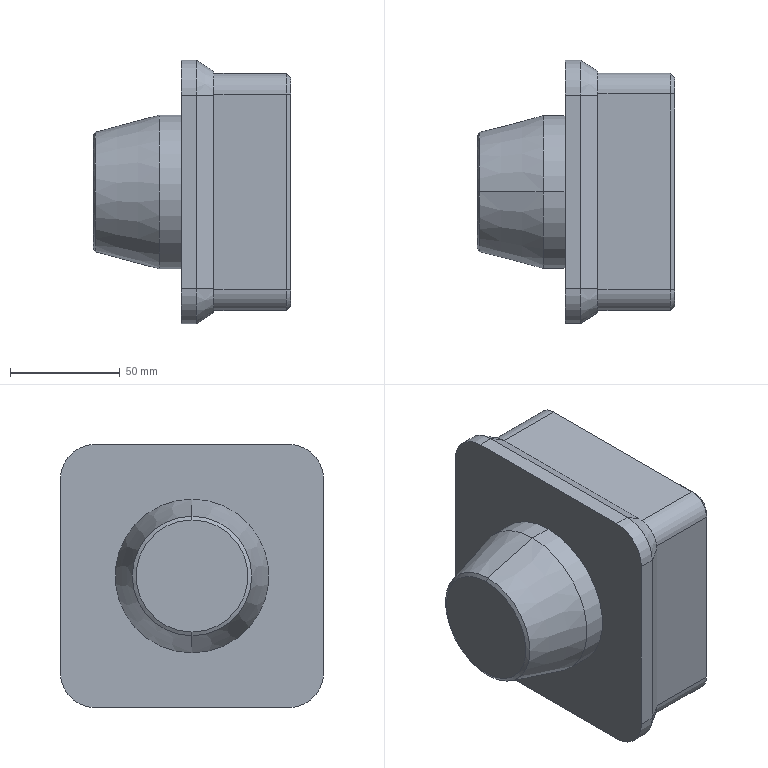Part | SolidWorks | features Chamfer 3, ICE 2, Revolution 1 | 1 solid | 42 faces | box 90 x 120 x 120 mm | volume 737957 mm3 | plane 20 | cone 12 | cylinder 10 | commonest cylinder face diameters 18.818 x4 32 x4 70 x2
STEP:
#1=CARTESIAN_POINT('',(0.,0.,25.547));
#2=VERTEX_POINT('',#1);
#3=CARTESIAN_POINT('',(0.,0.,-25.547));
#4=VERTEX_POINT('',#3);
#5=CARTESIAN_POINT('',(0.,0.,0.));
#6=DIRECTION('',(-1.,0.,0.));
#7=DIRECTION('',(0.,0.,1.));
#8=AXIS2_PLACEMENT_3D('',#5,#6,#7);
#9=CIRCLE('',#8,25.547);
#10=EDGE_CURVE('',#2,#4,#9,.T.);
#11=ORIENTED_EDGE('',*,*,#10,.F.);
#12=CARTESIAN_POINT('',(0.9659,0.,27.22));
#13=VERTEX_POINT('',#12);
#14=CARTESIAN_POINT('',(0.,0.,25.547));
#15=DIRECTION('',(0.5,0.,0.866));
#16=VECTOR('',#15,1000.);
#17=LINE('',#14,#16);
#18=EDGE_CURVE('',#2,#13,#17,.T.);
#19=ORIENTED_EDGE('',*,*,#18,.T.);
#20=CARTESIAN_POINT('',(0.9659,0.,-27.22));
#21=VERTEX_POINT('',#20);
#22=CARTESIAN_POINT('',(0.9659,0.,0.));
#23=DIRECTION('',(1.,0.,0.));
#24=DIRECTION('',(0.,0.,-1.));
#25=AXIS2_PLACEMENT_3D('',#22,#23,#24);
#26=CIRCLE('',#25,27.22);
#27=EDGE_CURVE('',#21,#13,#26,.T.);
#28=ORIENTED_EDGE('',*,*,#27,.F.);
#29=CARTESIAN_POINT('',(0.,0.,-25.547));
#30=DIRECTION('',(0.5,0.,-0.866));
#31=VECTOR('',#30,1000.);
#32=LINE('',#29,#31);
#33=EDGE_CURVE('',#4,#21,#32,.T.);
#34=ORIENTED_EDGE('',*,*,#33,.F.);
#35=EDGE_LOOP('',(#11,#19,#28,#34));
#36=FACE_OUTER_BOUND('',#35,.T.);
#37=CARTESIAN_POINT('',(0.,0.,0.));
#38=DIRECTION('',(1.,0.,0.));
#39=DIRECTION('',(0.,0.,-1.));
#40=AXIS2_PLACEMENT_3D('',#37,#38,#39);
#41=CONICAL_SURFACE('',#40,25.547,1.047);
#42=ADVANCED_FACE('',(#36),#41,.T.);
#43=ORIENTED_EDGE('',*,*,#27,.T.);
#44=CARTESIAN_POINT('',(30.,0.,35.));
#45=VERTEX_POINT('',#44);
#46=CARTESIAN_POINT('',(30.,0.,35.));
#47=DIRECTION('',(0.9659,0.,0.2588));
#48=VECTOR('',#47,1000.);
#49=LINE('',#46,#48);
#50=EDGE_CURVE('',#13,#45,#49,.T.);
#51=ORIENTED_EDGE('',*,*,#50,.T.);
#52=CARTESIAN_POINT('',(30.,0.,-35.));
#53=VERTEX_POINT('',#52);
#54=CARTESIAN_POINT('',(30.,0.,0.));
#55=DIRECTION('',(-1.,0.,0.));
#56=DIRECTION('',(0.,0.,1.));
#57=AXIS2_PLACEMENT_3D('',#54,#55,#56);
#58=CIRCLE('',#57,35.);
#59=EDGE_CURVE('',#45,#53,#58,.T.);
#60=ORIENTED_EDGE('',*,*,#59,.T.);
#61=CARTESIAN_POINT('',(30.,0.,-35.));
#62=DIRECTION('',(0.9659,0.,-0.2588));
#63=VECTOR('',#62,1000.);
#64=LINE('',#61,#63);
#65=EDGE_CURVE('',#21,#53,#64,.T.);
#66=ORIENTED_EDGE('',*,*,#65,.F.);
#67=EDGE_LOOP('',(#43,#51,#60,#66));
#68=FACE_OUTER_BOUND('',#67,.T.);
#69=CARTESIAN_POINT('',(30.,0.,0.));
#70=DIRECTION('',(1.,0.,0.));
#71=DIRECTION('',(0.,0.,-1.));
#72=AXIS2_PLACEMENT_3D('',#69,#70,#71);
#73=CONICAL_SURFACE('',#72,35.,0.2618);
#74=ADVANCED_FACE('',(#68),#73,.T.);
#75=CARTESIAN_POINT('',(40.,0.,35.));
#76=VERTEX_POINT('',#75);
#77=CARTESIAN_POINT('',(40.,0.,-35.));
#78=VERTEX_POINT('',#77);
#79=CARTESIAN_POINT('',(40.,0.,0.));
#80=DIRECTION('',(-1.,0.,0.));
#81=DIRECTION('',(0.,0.,1.));
#82=AXIS2_PLACEMENT_3D('',#79,#80,#81);
#83=CIRCLE('',#82,35.);
#84=EDGE_CURVE('',#76,#78,#83,.T.);
#85=ORIENTED_EDGE('',*,*,#84,.T.);
#86=CARTESIAN_POINT('',(0.,0.,-35.));
#87=DIRECTION('',(-1.,0.,0.));
#88=VECTOR('',#87,1000.);
#89=LINE('',#86,#88);
#90=EDGE_CURVE('',#78,#53,#89,.T.);
#91=ORIENTED_EDGE('',*,*,#90,.T.);
#92=ORIENTED_EDGE('',*,*,#59,.F.);
#93=CARTESIAN_POINT('',(0.,0.,35.));
#94=DIRECTION('',(-1.,0.,0.));
#95=VECTOR('',#94,1000.);
#96=LINE('',#93,#95);
#97=EDGE_CURVE('',#76,#45,#96,.T.);
#98=ORIENTED_EDGE('',*,*,#97,.F.);
#99=EDGE_LOOP('',(#85,#91,#92,#98));
#100=FACE_OUTER_BOUND('',#99,.T.);
#101=CARTESIAN_POINT('',(0.,0.,0.));
#102=DIRECTION('',(-1.,0.,0.));
#103=DIRECTION('',(0.,0.,1.));
#104=AXIS2_PLACEMENT_3D('',#101,#102,#103);
#105=CYLINDRICAL_SURFACE('',#104,35.);
#106=ADVANCED_FACE('',(#100),#105,.T.);
#107=CARTESIAN_POINT('',(55.,55.,44.));
#108=VERTEX_POINT('',#107);
#109=CARTESIAN_POINT('',(55.,44.,55.));
#110=VERTEX_POINT('',#109);
#111=CARTESIAN_POINT('',(55.,44.,44.));
#112=DIRECTION('',(1.,0.,0.));
#113=DIRECTION('',(0.,0.,1.));
#114=AXIS2_PLACEMENT_3D('',#111,#112,#113);
#115=CIRCLE('',#114,11.);
#116=EDGE_CURVE('',#108,#110,#115,.T.);
#117=ORIENTED_EDGE('',*,*,#116,.T.);
#118=CARTESIAN_POINT('',(55.,-44.,55.));
#119=VERTEX_POINT('',#118);
#120=CARTESIAN_POINT('',(55.,-44.,55.));
#121=DIRECTION('',(0.,-1.,0.));
#122=VECTOR('',#121,1000.);
#123=LINE('',#120,#122);
#124=EDGE_CURVE('',#110,#119,#123,.T.);
#125=ORIENTED_EDGE('',*,*,#124,.T.);
#126=CARTESIAN_POINT('',(55.,-55.,44.));
#127=VERTEX_POINT('',#126);
#128=CARTESIAN_POINT('',(55.,-44.,44.));
#129=DIRECTION('',(1.,0.,0.));
#130=DIRECTION('',(0.,0.,1.));
#131=AXIS2_PLACEMENT_3D('',#128,#129,#130);
#132=CIRCLE('',#131,11.);
#133=EDGE_CURVE('',#119,#127,#132,.T.);
#134=ORIENTED_EDGE('',*,*,#133,.T.);
#135=CARTESIAN_POINT('',(55.,-55.,-44.));
#136=VERTEX_POINT('',#135);
#137=CARTESIAN_POINT('',(55.,-55.,44.));
#138=DIRECTION('',(0.,0.,-1.));
#139=VECTOR('',#138,1000.);
#140=LINE('',#137,#139);
#141=EDGE_CURVE('',#127,#136,#140,.T.);
#142=ORIENTED_EDGE('',*,*,#141,.T.);
#143=CARTESIAN_POINT('',(55.,-44.,-55.));
#144=VERTEX_POINT('',#143);
#145=CARTESIAN_POINT('',(55.,-44.,-44.));
#146=DIRECTION('',(1.,0.,0.));
#147=DIRECTION('',(0.,0.,1.));
#148=AXIS2_PLACEMENT_3D('',#145,#146,#147);
#149=CIRCLE('',#148,11.);
#150=EDGE_CURVE('',#136,#144,#149,.T.);
#151=ORIENTED_EDGE('',*,*,#150,.T.);
#152=CARTESIAN_POINT('',(55.,44.,-55.));
#153=VERTEX_POINT('',#152);
#154=CARTESIAN_POINT('',(55.,-44.,-55.));
#155=DIRECTION('',(0.,1.,0.));
#156=VECTOR('',#155,1000.);
#157=LINE('',#154,#156);
#158=EDGE_CURVE('',#144,#153,#157,.T.);
#159=ORIENTED_EDGE('',*,*,#158,.T.);
#160=CARTESIAN_POINT('',(55.,55.,-44.));
#161=VERTEX_POINT('',#160);
#162=CARTESIAN_POINT('',(55.,44.,-44.));
#163=DIRECTION('',(1.,0.,0.));
#164=DIRECTION('',(0.,0.,1.));
#165=AXIS2_PLACEMENT_3D('',#162,#163,#164);
#166=CIRCLE('',#165,11.);
#167=EDGE_CURVE('',#153,#161,#166,.T.);
#168=ORIENTED_EDGE('',*,*,#167,.T.);
#169=CARTESIAN_POINT('',(55.,55.,44.));
#170=DIRECTION('',(0.,0.,1.));
#171=VECTOR('',#170,1000.);
#172=LINE('',#169,#171);
#173=EDGE_CURVE('',#161,#108,#172,.T.);
#174=ORIENTED_EDGE('',*,*,#173,.T.);
#175=EDGE_LOOP('',(#117,#125,#134,#142,#151,#159,#168,#174));
#176=FACE_OUTER_BOUND('',#175,.T.);
#177=CARTESIAN_POINT('',(55.,44.591,-54.));
#178=VERTEX_POINT('',#177);
#179=CARTESIAN_POINT('',(55.,54.,-44.591));
#180=VERTEX_POINT('',#179);
#181=CARTESIAN_POINT('',(55.,44.591,-44.591));
#182=DIRECTION('',(1.,0.,0.));
#183=DIRECTION('',(0.,0.,1.));
#184=AXIS2_PLACEMENT_3D('',#181,#182,#183);
#185=CIRCLE('',#184,9.409);
#186=EDGE_CURVE('',#178,#180,#185,.T.);
#187=ORIENTED_EDGE('',*,*,#186,.F.);
#188=CARTESIAN_POINT('',(55.,-44.591,-54.));
#189=VERTEX_POINT('',#188);
#190=CARTESIAN_POINT('',(55.,-44.591,-54.));
#191=DIRECTION('',(0.,1.,0.));
#192=VECTOR('',#191,1000.);
#193=LINE('',#190,#192);
#194=EDGE_CURVE('',#189,#178,#193,.T.);
#195=ORIENTED_EDGE('',*,*,#194,.F.);
#196=CARTESIAN_POINT('',(55.,-54.,-44.591));
#197=VERTEX_POINT('',#196);
#198=CARTESIAN_POINT('',(55.,-44.591,-44.591));
#199=DIRECTION('',(1.,0.,0.));
#200=DIRECTION('',(0.,0.,1.));
#201=AXIS2_PLACEMENT_3D('',#198,#199,#200);
#202=CIRCLE('',#201,9.409);
#203=EDGE_CURVE('',#197,#189,#202,.T.);
#204=ORIENTED_EDGE('',*,*,#203,.F.);
#205=CARTESIAN_POINT('',(55.,-54.,44.591));
#206=VERTEX_POINT('',#205);
#207=CARTESIAN_POINT('',(55.,-54.,44.591));
#208=DIRECTION('',(0.,0.,-1.));
#209=VECTOR('',#208,1000.);
#210=LINE('',#207,#209);
#211=EDGE_CURVE('',#206,#197,#210,.T.);
#212=ORIENTED_EDGE('',*,*,#211,.F.);
#213=CARTESIAN_POINT('',(55.,-44.591,54.));
#214=VERTEX_POINT('',#213);
#215=CARTESIAN_POINT('',(55.,-44.591,44.591));
#216=DIRECTION('',(1.,0.,0.));
#217=DIRECTION('',(0.,0.,1.));
#218=AXIS2_PLACEMENT_3D('',#215,#216,#217);
#219=CIRCLE('',#218,9.409);
#220=EDGE_CURVE('',#214,#206,#219,.T.);
#221=ORIENTED_EDGE('',*,*,#220,.F.);
#222=CARTESIAN_POINT('',(55.,44.591,54.));
#223=VERTEX_POINT('',#222);
#224=CARTESIAN_POINT('',(55.,-44.591,54.));
#225=DIRECTION('',(0.,-1.,0.));
#226=VECTOR('',#225,1000.);
#227=LINE('',#224,#226);
#228=EDGE_CURVE('',#223,#214,#227,.T.);
#229=ORIENTED_EDGE('',*,*,#228,.F.);
#230=CARTESIAN_POINT('',(55.,54.,44.591));
#231=VERTEX_POINT('',#230);
#232=CARTESIAN_POINT('',(55.,44.591,44.591));
#233=DIRECTION('',(1.,0.,0.));
#234=DIRECTION('',(0.,0.,1.));
#235=AXIS2_PLACEMENT_3D('',#232,#233,#234);
#236=CIRCLE('',#235,9.409);
#237=EDGE_CURVE('',#231,#223,#236,.T.);
#238=ORIENTED_EDGE('',*,*,#237,.F.);
#239=CARTESIAN_POINT('',(55.,54.,44.591));
#240=DIRECTION('',(0.,0.,1.));
#241=VECTOR('',#240,1000.);
#242=LINE('',#239,#241);
#243=EDGE_CURVE('',#180,#231,#242,.T.);
#244=ORIENTED_EDGE('',*,*,#243,.F.);
#245=EDGE_LOOP('',(#187,#195,#204,#212,#221,#229,#238,#244));
#246=FACE_BOUND('',#245,.T.);
#247=CARTESIAN_POINT('',(55.,-44.,44.));
#248=DIRECTION('',(-1.,0.,0.));
#249=DIRECTION('',(0.,0.,1.));
#250=AXIS2_PLACEMENT_3D('',#247,#248,#249);
#251=PLANE('',#250);
#252=ADVANCED_FACE('',(#176,#246),#251,.F.);
#253=ORIENTED_EDGE('',*,*,#90,.F.);
#254=CARTESIAN_POINT('',(40.,0.,0.));
#255=DIRECTION('',(-1.,0.,0.));
#256=DIRECTION('',(0.,0.,1.));
#257=AXIS2_PLACEMENT_3D('',#254,#255,#256);
#258=CIRCLE('',#257,35.);
#259=EDGE_CURVE('',#78,#76,#258,.T.);
#260=ORIENTED_EDGE('',*,*,#259,.T.);
#261=ORIENTED_EDGE('',*,*,#97,.T.);
#262=CARTESIAN_POINT('',(30.,0.,0.));
#263=DIRECTION('',(-1.,0.,0.));
#264=DIRECTION('',(0.,0.,1.));
#265=AXIS2_PLACEMENT_3D('',#262,#263,#264);
#266=CIRCLE('',#265,35.);
#267=EDGE_CURVE('',#53,#45,#266,.T.);
#268=ORIENTED_EDGE('',*,*,#267,.F.);
#269=EDGE_LOOP('',(#253,#260,#261,#268));
#270=FACE_OUTER_BOUND('',#269,.T.);
#271=CARTESIAN_POINT('',(0.,0.,0.));
#272=DIRECTION('',(-1.,0.,0.));
#273=DIRECTION('',(0.,0.,1.));
#274=AXIS2_PLACEMENT_3D('',#271,#272,#273);
#275=CYLINDRICAL_SURFACE('',#274,35.);
#276=ADVANCED_FACE('',(#270),#275,.T.);
#277=ORIENTED_EDGE('',*,*,#50,.F.);
#278=CARTESIAN_POINT('',(0.9659,0.,0.));
#279=DIRECTION('',(1.,0.,0.));
#280=DIRECTION('',(0.,0.,-1.));
#281=AXIS2_PLACEMENT_3D('',#278,#279,#280);
#282=CIRCLE('',#281,27.22);
#283=EDGE_CURVE('',#13,#21,#282,.T.);
#284=ORIENTED_EDGE('',*,*,#283,.T.);
#285=ORIENTED_EDGE('',*,*,#65,.T.);
#286=ORIENTED_EDGE('',*,*,#267,.T.);
#287=EDGE_LOOP('',(#277,#284,#285,#286));
#288=FACE_OUTER_BOUND('',#287,.T.);
#289=CARTESIAN_POINT('',(30.,0.,0.));
#290=DIRECTION('',(1.,0.,0.));
#291=DIRECTION('',(0.,0.,-1.));
#292=AXIS2_PLACEMENT_3D('',#289,#290,#291);
#293=CONICAL_SURFACE('',#292,35.,0.2618);
#294=ADVANCED_FACE('',(#288),#293,.T.);
#295=CARTESIAN_POINT('',(0.,0.,0.));
#296=DIRECTION('',(-1.,0.,0.));
#297=DIRECTION('',(0.,0.,1.));
#298=AXIS2_PLACEMENT_3D('',#295,#296,#297);
#299=CIRCLE('',#298,25.547);
#300=EDGE_CURVE('',#4,#2,#299,.T.);
#301=ORIENTED_EDGE('',*,*,#300,.T.);
#302=ORIENTED_EDGE('',*,*,#10,.T.);
#303=EDGE_LOOP('',(#301,#302));
#304=FACE_OUTER_BOUND('',#303,.T.);
#305=CARTESIAN_POINT('',(0.,0.,0.));
#306=DIRECTION('',(-1.,0.,0.));
#307=DIRECTION('',(0.,0.,1.));
#308=AXIS2_PLACEMENT_3D('',#305,#306,#307);
#309=PLANE('',#308);
#310=ADVANCED_FACE('',(#304),#309,.T.);
#311=CARTESIAN_POINT('',(47.,-60.,44.));
#312=VERTEX_POINT('',#311);
#313=CARTESIAN_POINT('',(40.,-60.,44.));
#314=VERTEX_POINT('',#313);
#315=CARTESIAN_POINT('',(55.,-60.,44.));
#316=DIRECTION('',(-1.,0.,0.));
#317=VECTOR('',#316,1000.);
#318=LINE('',#315,#317);
#319=EDGE_CURVE('',#312,#314,#318,.T.);
#320=ORIENTED_EDGE('',*,*,#319,.F.);
#321=CARTESIAN_POINT('',(47.,-44.,60.));
#322=VERTEX_POINT('',#321);
#323=CARTESIAN_POINT('',(47.,-44.,44.));
#324=DIRECTION('',(-1.,0.,0.));
#325=DIRECTION('',(0.,0.,1.));
#326=AXIS2_PLACEMENT_3D('',#323,#324,#325);
#327=CIRCLE('',#326,16.);
#328=EDGE_CURVE('',#312,#322,#327,.T.);
#329=ORIENTED_EDGE('',*,*,#328,.T.);
#330=CARTESIAN_POINT('',(40.,-44.,60.));
#331=VERTEX_POINT('',#330);
#332=CARTESIAN_POINT('',(55.,-44.,60.));
#333=DIRECTION('',(-1.,0.,0.));
#334=VECTOR('',#333,1000.);
#335=LINE('',#332,#334);
#336=EDGE_CURVE('',#322,#331,#335,.T.);
#337=ORIENTED_EDGE('',*,*,#336,.T.);
#338=CARTESIAN_POINT('',(40.,-44.,44.));
#339=DIRECTION('',(1.,0.,0.));
#340=DIRECTION('',(0.,0.,1.));
#341=AXIS2_PLACEMENT_3D('',#338,#339,#340);
#342=CIRCLE('',#341,16.);
#343=EDGE_CURVE('',#331,#314,#342,.T.);
#344=ORIENTED_EDGE('',*,*,#343,.T.);
#345=EDGE_LOOP('',(#320,#329,#337,#344));
#346=FACE_OUTER_BOUND('',#345,.T.);
#347=CARTESIAN_POINT('',(55.,-44.,44.));
#348=DIRECTION('',(-1.,0.,0.));
#349=DIRECTION('',(0.,0.,1.));
#350=AXIS2_PLACEMENT_3D('',#347,#348,#349);
#351=CYLINDRICAL_SURFACE('',#350,16.);
#352=ADVANCED_FACE('',(#346),#351,.T.);
#353=CARTESIAN_POINT('',(47.,-60.,-44.));
#354=VERTEX_POINT('',#353);
#355=CARTESIAN_POINT('',(40.,-60.,-44.));
#356=VERTEX_POINT('',#355);
#357=CARTESIAN_POINT('',(55.,-60.,-44.));
#358=DIRECTION('',(-1.,0.,0.));
#359=VECTOR('',#358,1000.);
#360=LINE('',#357,#359);
#361=EDGE_CURVE('',#354,#356,#360,.T.);
#362=ORIENTED_EDGE('',*,*,#361,.F.);
#363=CARTESIAN_POINT('',(47.,-60.,44.));
#364=DIRECTION('',(0.,0.,1.));
#365=VECTOR('',#364,1000.);
#366=LINE('',#363,#365);
#367=EDGE_CURVE('',#354,#312,#366,.T.);
#368=ORIENTED_EDGE('',*,*,#367,.T.);
#369=ORIENTED_EDGE('',*,*,#319,.T.);
#370=CARTESIAN_POINT('',(40.,-60.,44.));
#371=DIRECTION('',(0.,0.,-1.));
#372=VECTOR('',#371,1000.);
#373=LINE('',#370,#372);
#374=EDGE_CURVE('',#314,#356,#373,.T.);
#375=ORIENTED_EDGE('',*,*,#374,.T.);
#376=EDGE_LOOP('',(#362,#368,#369,#375));
#377=FACE_OUTER_BOUND('',#376,.T.);
#378=CARTESIAN_POINT('',(55.,-60.,44.));
#379=DIRECTION('',(0.,1.,0.));
#380=DIRECTION('',(0.,0.,1.));
#381=AXIS2_PLACEMENT_3D('',#378,#379,#380);
#382=PLANE('',#381);
#383=ADVANCED_FACE('',(#377),#382,.F.);
#384=CARTESIAN_POINT('',(47.,-44.,-60.));
#385=VERTEX_POINT('',#384);
#386=CARTESIAN_POINT('',(40.,-44.,-60.));
#387=VERTEX_POINT('',#386);
#388=CARTESIAN_POINT('',(55.,-44.,-60.));
#389=DIRECTION('',(-1.,0.,0.));
#390=VECTOR('',#389,1000.);
#391=LINE('',#388,#390);
#392=EDGE_CURVE('',#385,#387,#391,.T.);
#393=ORIENTED_EDGE('',*,*,#392,.F.);
#394=CARTESIAN_POINT('',(47.,-44.,-44.));
#395=DIRECTION('',(-1.,0.,0.));
#396=DIRECTION('',(0.,0.,1.));
#397=AXIS2_PLACEMENT_3D('',#394,#395,#396);
#398=CIRCLE('',#397,16.);
#399=EDGE_CURVE('',#385,#354,#398,.T.);
#400=ORIENTED_EDGE('',*,*,#399,.T.);
#401=ORIENTED_EDGE('',*,*,#361,.T.);
#402=CARTESIAN_POINT('',(40.,-44.,-44.));
#403=DIRECTION('',(1.,0.,0.));
#404=DIRECTION('',(0.,0.,-1.));
#405=AXIS2_PLACEMENT_3D('',#402,#403,#404);
#406=CIRCLE('',#405,16.);
#407=EDGE_CURVE('',#356,#387,#406,.T.);
#408=ORIENTED_EDGE('',*,*,#407,.T.);
#409=EDGE_LOOP('',(#393,#400,#401,#408));
#410=FACE_OUTER_BOUND('',#409,.T.);
#411=CARTESIAN_POINT('',(55.,-44.,-44.));
#412=DIRECTION('',(-1.,0.,0.));
#413=DIRECTION('',(0.,0.,1.));
#414=AXIS2_PLACEMENT_3D('',#411,#412,#413);
#415=CYLINDRICAL_SURFACE('',#414,16.);
#416=ADVANCED_FACE('',(#410),#415,.T.);
#417=CARTESIAN_POINT('',(47.,44.,-60.));
#418=VERTEX_POINT('',#417);
#419=CARTESIAN_POINT('',(40.,44.,-60.));
#420=VERTEX_POINT('',#419);
#421=CARTESIAN_POINT('',(55.,44.,-60.));
#422=DIRECTION('',(-1.,0.,0.));
#423=VECTOR('',#422,1000.);
#424=LINE('',#421,#423);
#425=EDGE_CURVE('',#418,#420,#424,.T.);
#426=ORIENTED_EDGE('',*,*,#425,.F.);
#427=CARTESIAN_POINT('',(47.,-44.,-60.));
#428=DIRECTION('',(0.,-1.,0.));
#429=VECTOR('',#428,1000.);
#430=LINE('',#427,#429);
#431=EDGE_CURVE('',#418,#385,#430,.T.);
#432=ORIENTED_EDGE('',*,*,#431,.T.);
#433=ORIENTED_EDGE('',*,*,#392,.T.);
#434=CARTESIAN_POINT('',(40.,-44.,-60.));
#435=DIRECTION('',(0.,1.,0.));
#436=VECTOR('',#435,1000.);
#437=LINE('',#434,#436);
#438=EDGE_CURVE('',#387,#420,#437,.T.);
#439=ORIENTED_EDGE('',*,*,#438,.T.);
#440=EDGE_LOOP('',(#426,#432,#433,#439));
#441=FACE_OUTER_BOUND('',#440,.T.);
#442=CARTESIAN_POINT('',(55.,-44.,-60.));
#443=DIRECTION('',(0.,0.,1.));
#444=DIRECTION('',(1.,0.,0.));
#445=AXIS2_PLACEMENT_3D('',#442,#443,#444);
#446=PLANE('',#445);
#447=ADVANCED_FACE('',(#441),#446,.F.);
#448=CARTESIAN_POINT('',(47.,60.,-44.));
#449=VERTEX_POINT('',#448);
#450=CARTESIAN_POINT('',(40.,60.,-44.));
#451=VERTEX_POINT('',#450);
#452=CARTESIAN_POINT('',(55.,60.,-44.));
#453=DIRECTION('',(-1.,0.,0.));
#454=VECTOR('',#453,1000.);
#455=LINE('',#452,#454);
#456=EDGE_CURVE('',#449,#451,#455,.T.);
#457=ORIENTED_EDGE('',*,*,#456,.F.);
#458=CARTESIAN_POINT('',(47.,44.,-44.));
#459=DIRECTION('',(-1.,0.,0.));
#460=DIRECTION('',(0.,0.,1.));
#461=AXIS2_PLACEMENT_3D('',#458,#459,#460);
#462=CIRCLE('',#461,16.);
#463=EDGE_CURVE('',#449,#418,#462,.T.);
#464=ORIENTED_EDGE('',*,*,#463,.T.);
#465=ORIENTED_EDGE('',*,*,#425,.T.);
#466=CARTESIAN_POINT('',(40.,44.,-44.));
#467=DIRECTION('',(1.,0.,0.));
#468=DIRECTION('',(0.,0.,1.));
#469=AXIS2_PLACEMENT_3D('',#466,#467,#468);
#470=CIRCLE('',#469,16.);
#471=EDGE_CURVE('',#420,#451,#470,.T.);
#472=ORIENTED_EDGE('',*,*,#471,.T.);
#473=EDGE_LOOP('',(#457,#464,#465,#472));
#474=FACE_OUTER_BOUND('',#473,.T.);
#475=CARTESIAN_POINT('',(55.,44.,-44.));
#476=DIRECTION('',(-1.,0.,0.));
#477=DIRECTION('',(0.,0.,1.));
#478=AXIS2_PLACEMENT_3D('',#475,#476,#477);
#479=CYLINDRICAL_SURFACE('',#478,16.);
#480=ADVANCED_FACE('',(#474),#479,.T.);
#481=CARTESIAN_POINT('',(47.,60.,44.));
#482=VERTEX_POINT('',#481);
#483=CARTESIAN_POINT('',(40.,60.,44.));
#484=VERTEX_POINT('',#483);
#485=CARTESIAN_POINT('',(55.,60.,44.));
#486=DIRECTION('',(-1.,0.,0.));
#487=VECTOR('',#486,1000.);
#488=LINE('',#485,#487);
#489=EDGE_CURVE('',#482,#484,#488,.T.);
#490=ORIENTED_EDGE('',*,*,#489,.F.);
#491=CARTESIAN_POINT('',(47.,60.,44.));
#492=DIRECTION('',(0.,0.,-1.));
#493=VECTOR('',#492,1000.);
#494=LINE('',#491,#493);
#495=EDGE_CURVE('',#482,#449,#494,.T.);
#496=ORIENTED_EDGE('',*,*,#495,.T.);
#497=ORIENTED_EDGE('',*,*,#456,.T.);
#498=CARTESIAN_POINT('',(40.,60.,44.));
#499=DIRECTION('',(0.,0.,1.));
#500=VECTOR('',#499,1000.);
#501=LINE('',#498,#500);
#502=EDGE_CURVE('',#451,#484,#501,.T.);
#503=ORIENTED_EDGE('',*,*,#502,.T.);
#504=EDGE_LOOP('',(#490,#496,#497,#503));
#505=FACE_OUTER_BOUND('',#504,.T.);
#506=CARTESIAN_POINT('',(55.,60.,44.));
#507=DIRECTION('',(0.,-1.,0.));
#508=DIRECTION('',(0.,0.,-1.));
#509=AXIS2_PLACEMENT_3D('',#506,#507,#508);
#510=PLANE('',#509);
#511=ADVANCED_FACE('',(#505),#510,.F.);
#512=CARTESIAN_POINT('',(47.,44.,60.));
#513=VERTEX_POINT('',#512);
#514=CARTESIAN_POINT('',(40.,44.,60.));
#515=VERTEX_POINT('',#514);
#516=CARTESIAN_POINT('',(55.,44.,60.));
#517=DIRECTION('',(-1.,0.,0.));
#518=VECTOR('',#517,1000.);
#519=LINE('',#516,#518);
#520=EDGE_CURVE('',#513,#515,#519,.T.);
#521=ORIENTED_EDGE('',*,*,#520,.F.);
#522=CARTESIAN_POINT('',(47.,44.,44.));
#523=DIRECTION('',(-1.,0.,0.));
#524=DIRECTION('',(0.,0.,1.));
#525=AXIS2_PLACEMENT_3D('',#522,#523,#524);
#526=CIRCLE('',#525,16.);
#527=EDGE_CURVE('',#513,#482,#526,.T.);
#528=ORIENTED_EDGE('',*,*,#527,.T.);
#529=ORIENTED_EDGE('',*,*,#489,.T.);
#530=CARTESIAN_POINT('',(40.,44.,44.));
#531=DIRECTION('',(1.,0.,0.));
#532=DIRECTION('',(0.,0.,-1.));
#533=AXIS2_PLACEMENT_3D('',#530,#531,#532);
#534=CIRCLE('',#533,16.);
#535=EDGE_CURVE('',#484,#515,#534,.T.);
#536=ORIENTED_EDGE('',*,*,#535,.T.);
#537=EDGE_LOOP('',(#521,#528,#529,#536));
#538=FACE_OUTER_BOUND('',#537,.T.);
#539=CARTESIAN_POINT('',(55.,44.,44.));
#540=DIRECTION('',(-1.,0.,0.));
#541=DIRECTION('',(0.,0.,1.));
#542=AXIS2_PLACEMENT_3D('',#539,#540,#541);
#543=CYLINDRICAL_SURFACE('',#542,16.);
#544=ADVANCED_FACE('',(#538),#543,.T.);
#545=ORIENTED_EDGE('',*,*,#336,.F.);
#546=CARTESIAN_POINT('',(47.,-44.,60.));
#547=DIRECTION('',(0.,1.,0.));
#548=VECTOR('',#547,1000.);
#549=LINE('',#546,#548);
#550=EDGE_CURVE('',#322,#513,#549,.T.);
#551=ORIENTED_EDGE('',*,*,#550,.T.);
#552=ORIENTED_EDGE('',*,*,#520,.T.);
#553=CARTESIAN_POINT('',(40.,-44.,60.));
#554=DIRECTION('',(0.,-1.,0.));
#555=VECTOR('',#554,1000.);
#556=LINE('',#553,#555);
#557=EDGE_CURVE('',#515,#331,#556,.T.);
#558=ORIENTED_EDGE('',*,*,#557,.T.);
#559=EDGE_LOOP('',(#545,#551,#552,#558));
#560=FACE_OUTER_BOUND('',#559,.T.);
#561=CARTESIAN_POINT('',(55.,-44.,60.));
#562=DIRECTION('',(0.,0.,-1.));
#563=DIRECTION('',(-1.,0.,0.));
#564=AXIS2_PLACEMENT_3D('',#561,#562,#563);
#565=PLANE('',#564);
#566=ADVANCED_FACE('',(#560),#565,.F.);
#567=ORIENTED_EDGE('',*,*,#84,.F.);
#568=ORIENTED_EDGE('',*,*,#259,.F.);
#569=EDGE_LOOP('',(#567,#568));
#570=FACE_BOUND('',#569,.T.);
#571=ORIENTED_EDGE('',*,*,#343,.F.);
#572=ORIENTED_EDGE('',*,*,#557,.F.);
#573=ORIENTED_EDGE('',*,*,#535,.F.);
#574=ORIENTED_EDGE('',*,*,#502,.F.);
#575=ORIENTED_EDGE('',*,*,#471,.F.);
#576=ORIENTED_EDGE('',*,*,#438,.F.);
#577=ORIENTED_EDGE('',*,*,#407,.F.);
#578=ORIENTED_EDGE('',*,*,#374,.F.);
#579=EDGE_LOOP('',(#571,#572,#573,#574,#575,#576,#577,#578));
#580=FACE_OUTER_BOUND('',#579,.T.);
#581=CARTESIAN_POINT('',(40.,-44.,44.));
#582=DIRECTION('',(-1.,0.,0.));
#583=DIRECTION('',(0.,0.,1.));
#584=AXIS2_PLACEMENT_3D('',#581,#582,#583);
#585=PLANE('',#584);
#586=ADVANCED_FACE('',(#570,#580),#585,.T.);
#587=CARTESIAN_POINT('',(47.,-44.,-60.));
#588=DIRECTION('',(0.848,0.,0.53));
#589=VECTOR('',#588,1000.);
#590=LINE('',#587,#589);
#591=EDGE_CURVE('',#385,#144,#590,.T.);
#592=ORIENTED_EDGE('',*,*,#591,.F.);
#593=ORIENTED_EDGE('',*,*,#431,.F.);
#594=CARTESIAN_POINT('',(55.,44.,-55.));
#595=DIRECTION('',(-0.848,0.,-0.53));
#596=VECTOR('',#595,1000.);
#597=LINE('',#594,#596);
#598=EDGE_CURVE('',#153,#418,#597,.T.);
#599=ORIENTED_EDGE('',*,*,#598,.F.);
#600=ORIENTED_EDGE('',*,*,#158,.F.);
#601=EDGE_LOOP('',(#592,#593,#599,#600));
#602=FACE_OUTER_BOUND('',#601,.T.);
#603=CARTESIAN_POINT('',(55.,-44.,-55.));
#604=DIRECTION('',(-0.53,0.,0.848));
#605=DIRECTION('',(0.,1.,0.));
#606=AXIS2_PLACEMENT_3D('',#603,#604,#605);
#607=PLANE('',#606);
#608=ADVANCED_FACE('',(#602),#607,.F.);
#609=ORIENTED_EDGE('',*,*,#598,.T.);
#610=ORIENTED_EDGE('',*,*,#463,.F.);
#611=CARTESIAN_POINT('',(55.,55.,-44.));
#612=DIRECTION('',(-0.848,0.53,0.));
#613=VECTOR('',#612,1000.);
#614=LINE('',#611,#613);
#615=EDGE_CURVE('',#161,#449,#614,.T.);
#616=ORIENTED_EDGE('',*,*,#615,.F.);
#617=ORIENTED_EDGE('',*,*,#167,.F.);
#618=EDGE_LOOP('',(#609,#610,#616,#617));
#619=FACE_OUTER_BOUND('',#618,.T.);
#620=CARTESIAN_POINT('',(55.,44.,-44.));
#621=DIRECTION('',(-1.,0.,0.));
#622=DIRECTION('',(0.,0.,1.));
#623=AXIS2_PLACEMENT_3D('',#620,#621,#622);
#624=CONICAL_SURFACE('',#623,11.,0.5586);
#625=ADVANCED_FACE('',(#619),#624,.T.);
#626=ORIENTED_EDGE('',*,*,#591,.T.);
#627=ORIENTED_EDGE('',*,*,#150,.F.);
#628=CARTESIAN_POINT('',(47.,-60.,-44.));
#629=DIRECTION('',(0.848,0.53,0.));
#630=VECTOR('',#629,1000.);
#631=LINE('',#628,#630);
#632=EDGE_CURVE('',#354,#136,#631,.T.);
#633=ORIENTED_EDGE('',*,*,#632,.F.);
#634=ORIENTED_EDGE('',*,*,#399,.F.);
#635=EDGE_LOOP('',(#626,#627,#633,#634));
#636=FACE_OUTER_BOUND('',#635,.T.);
#637=CARTESIAN_POINT('',(55.,-44.,-44.));
#638=DIRECTION('',(-1.,0.,0.));
#639=DIRECTION('',(0.,0.,1.));
#640=AXIS2_PLACEMENT_3D('',#637,#638,#639);
#641=CONICAL_SURFACE('',#640,11.,0.5586);
#642=ADVANCED_FACE('',(#636),#641,.T.);
#643=ORIENTED_EDGE('',*,*,#615,.T.);
#644=ORIENTED_EDGE('',*,*,#495,.F.);
#645=CARTESIAN_POINT('',(55.,55.,44.));
#646=DIRECTION('',(-0.848,0.53,0.));
#647=VECTOR('',#646,1000.);
#648=LINE('',#645,#647);
#649=EDGE_CURVE('',#108,#482,#648,.T.);
#650=ORIENTED_EDGE('',*,*,#649,.F.);
#651=ORIENTED_EDGE('',*,*,#173,.F.);
#652=EDGE_LOOP('',(#643,#644,#650,#651));
#653=FACE_OUTER_BOUND('',#652,.T.);
#654=CARTESIAN_POINT('',(55.,55.,44.));
#655=DIRECTION('',(-0.53,-0.848,0.));
#656=DIRECTION('',(0.,0.,1.));
#657=AXIS2_PLACEMENT_3D('',#654,#655,#656);
#658=PLANE('',#657);
#659=ADVANCED_FACE('',(#653),#658,.F.);
#660=ORIENTED_EDGE('',*,*,#632,.T.);
#661=ORIENTED_EDGE('',*,*,#141,.F.);
#662=CARTESIAN_POINT('',(47.,-60.,44.));
#663=DIRECTION('',(0.848,0.53,0.));
#664=VECTOR('',#663,1000.);
#665=LINE('',#662,#664);
#666=EDGE_CURVE('',#312,#127,#665,.T.);
#667=ORIENTED_EDGE('',*,*,#666,.F.);
#668=ORIENTED_EDGE('',*,*,#367,.F.);
#669=EDGE_LOOP('',(#660,#661,#667,#668));
#670=FACE_OUTER_BOUND('',#669,.T.);
#671=CARTESIAN_POINT('',(55.,-55.,44.));
#672=DIRECTION('',(-0.53,0.848,0.));
#673=DIRECTION('',(0.,0.,-1.));
#674=AXIS2_PLACEMENT_3D('',#671,#672,#673);
#675=PLANE('',#674);
#676=ADVANCED_FACE('',(#670),#675,.F.);
#677=ORIENTED_EDGE('',*,*,#649,.T.);
#678=ORIENTED_EDGE('',*,*,#527,.F.);
#679=CARTESIAN_POINT('',(55.,44.,55.));
#680=DIRECTION('',(-0.848,0.,0.53));
#681=VECTOR('',#680,1000.);
#682=LINE('',#679,#681);
#683=EDGE_CURVE('',#110,#513,#682,.T.);
#684=ORIENTED_EDGE('',*,*,#683,.F.);
#685=ORIENTED_EDGE('',*,*,#116,.F.);
#686=EDGE_LOOP('',(#677,#678,#684,#685));
#687=FACE_OUTER_BOUND('',#686,.T.);
#688=CARTESIAN_POINT('',(55.,44.,44.));
#689=DIRECTION('',(-1.,0.,0.));
#690=DIRECTION('',(0.,0.,1.));
#691=AXIS2_PLACEMENT_3D('',#688,#689,#690);
#692=CONICAL_SURFACE('',#691,11.,0.5586);
#693=ADVANCED_FACE('',(#687),#692,.T.);
#694=ORIENTED_EDGE('',*,*,#666,.T.);
#695=ORIENTED_EDGE('',*,*,#133,.F.);
#696=CARTESIAN_POINT('',(47.,-44.,60.));
#697=DIRECTION('',(0.848,0.,-0.53));
#698=VECTOR('',#697,1000.);
#699=LINE('',#696,#698);
#700=EDGE_CURVE('',#322,#119,#699,.T.);
#701=ORIENTED_EDGE('',*,*,#700,.F.);
#702=ORIENTED_EDGE('',*,*,#328,.F.);
#703=EDGE_LOOP('',(#694,#695,#701,#702));
#704=FACE_OUTER_BOUND('',#703,.T.);
#705=CARTESIAN_POINT('',(55.,-44.,44.));
#706=DIRECTION('',(-1.,0.,0.));
#707=DIRECTION('',(0.,0.,1.));
#708=AXIS2_PLACEMENT_3D('',#705,#706,#707);
#709=CONICAL_SURFACE('',#708,11.,0.5586);
#710=ADVANCED_FACE('',(#704),#709,.T.);
#711=ORIENTED_EDGE('',*,*,#683,.T.);
#712=ORIENTED_EDGE('',*,*,#550,.F.);
#713=ORIENTED_EDGE('',*,*,#700,.T.);
#714=ORIENTED_EDGE('',*,*,#124,.F.);
#715=EDGE_LOOP('',(#711,#712,#713,#714));
#716=FACE_OUTER_BOUND('',#715,.T.);
#717=CARTESIAN_POINT('',(55.,-44.,55.));
#718=DIRECTION('',(-0.53,0.,-0.848));
#719=DIRECTION('',(0.,-1.,0.));
#720=AXIS2_PLACEMENT_3D('',#717,#718,#719);
#721=PLANE('',#720);
#722=ADVANCED_FACE('',(#716),#721,.F.);
#723=CARTESIAN_POINT('',(88.,54.,-44.591));
#724=VERTEX_POINT('',#723);
#725=CARTESIAN_POINT('',(90.,54.,-44.591));
#726=DIRECTION('',(-1.,0.,0.));
#727=VECTOR('',#726,1000.);
#728=LINE('',#725,#727);
#729=EDGE_CURVE('',#724,#180,#728,.T.);
#730=ORIENTED_EDGE('',*,*,#729,.F.);
#731=CARTESIAN_POINT('',(88.,44.591,-54.));
#732=VERTEX_POINT('',#731);
#733=CARTESIAN_POINT('',(88.,44.591,-44.591));
#734=DIRECTION('',(-1.,0.,0.));
#735=DIRECTION('',(0.,0.,1.));
#736=AXIS2_PLACEMENT_3D('',#733,#734,#735);
#737=CIRCLE('',#736,9.409);
#738=EDGE_CURVE('',#724,#732,#737,.T.);
#739=ORIENTED_EDGE('',*,*,#738,.T.);
#740=CARTESIAN_POINT('',(90.,44.591,-54.));
#741=DIRECTION('',(-1.,0.,0.));
#742=VECTOR('',#741,1000.);
#743=LINE('',#740,#742);
#744=EDGE_CURVE('',#732,#178,#743,.T.);
#745=ORIENTED_EDGE('',*,*,#744,.T.);
#746=ORIENTED_EDGE('',*,*,#186,.T.);
#747=EDGE_LOOP('',(#730,#739,#745,#746));
#748=FACE_OUTER_BOUND('',#747,.T.);
#749=CARTESIAN_POINT('',(90.,44.591,-44.591));
#750=DIRECTION('',(-1.,0.,0.));
#751=DIRECTION('',(0.,0.,1.));
#752=AXIS2_PLACEMENT_3D('',#749,#750,#751);
#753=CYLINDRICAL_SURFACE('',#752,9.409);
#754=ADVANCED_FACE('',(#748),#753,.T.);
#755=CARTESIAN_POINT('',(88.,54.,44.591));
#756=VERTEX_POINT('',#755);
#757=CARTESIAN_POINT('',(90.,54.,44.591));
#758=DIRECTION('',(-1.,0.,0.));
#759=VECTOR('',#758,1000.);
#760=LINE('',#757,#759);
#761=EDGE_CURVE('',#756,#231,#760,.T.);
#762=ORIENTED_EDGE('',*,*,#761,.F.);
#763=CARTESIAN_POINT('',(88.,54.,44.591));
#764=DIRECTION('',(0.,0.,-1.));
#765=VECTOR('',#764,1000.);
#766=LINE('',#763,#765);
#767=EDGE_CURVE('',#756,#724,#766,.T.);
#768=ORIENTED_EDGE('',*,*,#767,.T.);
#769=ORIENTED_EDGE('',*,*,#729,.T.);
#770=ORIENTED_EDGE('',*,*,#243,.T.);
#771=EDGE_LOOP('',(#762,#768,#769,#770));
#772=FACE_OUTER_BOUND('',#771,.T.);
#773=CARTESIAN_POINT('',(90.,54.,44.591));
#774=DIRECTION('',(0.,-1.,0.));
#775=DIRECTION('',(0.,0.,-1.));
#776=AXIS2_PLACEMENT_3D('',#773,#774,#775);
#777=PLANE('',#776);
#778=ADVANCED_FACE('',(#772),#777,.F.);
#779=CARTESIAN_POINT('',(88.,44.591,54.));
#780=VERTEX_POINT('',#779);
#781=CARTESIAN_POINT('',(90.,44.591,54.));
#782=DIRECTION('',(-1.,0.,0.));
#783=VECTOR('',#782,1000.);
#784=LINE('',#781,#783);
#785=EDGE_CURVE('',#780,#223,#784,.T.);
#786=ORIENTED_EDGE('',*,*,#785,.F.);
#787=CARTESIAN_POINT('',(88.,44.591,44.591));
#788=DIRECTION('',(-1.,0.,0.));
#789=DIRECTION('',(0.,0.,1.));
#790=AXIS2_PLACEMENT_3D('',#787,#788,#789);
#791=CIRCLE('',#790,9.409);
#792=EDGE_CURVE('',#780,#756,#791,.T.);
#793=ORIENTED_EDGE('',*,*,#792,.T.);
#794=ORIENTED_EDGE('',*,*,#761,.T.);
#795=ORIENTED_EDGE('',*,*,#237,.T.);
#796=EDGE_LOOP('',(#786,#793,#794,#795));
#797=FACE_OUTER_BOUND('',#796,.T.);
#798=CARTESIAN_POINT('',(90.,44.591,44.591));
#799=DIRECTION('',(-1.,0.,0.));
#800=DIRECTION('',(0.,0.,1.));
#801=AXIS2_PLACEMENT_3D('',#798,#799,#800);
#802=CYLINDRICAL_SURFACE('',#801,9.409);
#803=ADVANCED_FACE('',(#797),#802,.T.);
#804=CARTESIAN_POINT('',(88.,-44.591,54.));
#805=VERTEX_POINT('',#804);
#806=CARTESIAN_POINT('',(90.,-44.591,54.));
#807=DIRECTION('',(-1.,0.,0.));
#808=VECTOR('',#807,1000.);
#809=LINE('',#806,#808);
#810=EDGE_CURVE('',#805,#214,#809,.T.);
#811=ORIENTED_EDGE('',*,*,#810,.F.);
#812=CARTESIAN_POINT('',(88.,-44.591,54.));
#813=DIRECTION('',(0.,1.,0.));
#814=VECTOR('',#813,1000.);
#815=LINE('',#812,#814);
#816=EDGE_CURVE('',#805,#780,#815,.T.);
#817=ORIENTED_EDGE('',*,*,#816,.T.);
#818=ORIENTED_EDGE('',*,*,#785,.T.);
#819=ORIENTED_EDGE('',*,*,#228,.T.);
#820=EDGE_LOOP('',(#811,#817,#818,#819));
#821=FACE_OUTER_BOUND('',#820,.T.);
#822=CARTESIAN_POINT('',(90.,-44.591,54.));
#823=DIRECTION('',(0.,0.,-1.));
#824=DIRECTION('',(-1.,0.,0.));
#825=AXIS2_PLACEMENT_3D('',#822,#823,#824);
#826=PLANE('',#825);
#827=ADVANCED_FACE('',(#821),#826,.F.);
#828=CARTESIAN_POINT('',(88.,-54.,44.591));
#829=VERTEX_POINT('',#828);
#830=CARTESIAN_POINT('',(90.,-54.,44.591));
#831=DIRECTION('',(-1.,0.,0.));
#832=VECTOR('',#831,1000.);
#833=LINE('',#830,#832);
#834=EDGE_CURVE('',#829,#206,#833,.T.);
#835=ORIENTED_EDGE('',*,*,#834,.F.);
#836=CARTESIAN_POINT('',(88.,-44.591,44.591));
#837=DIRECTION('',(-1.,0.,0.));
#838=DIRECTION('',(0.,0.,1.));
#839=AXIS2_PLACEMENT_3D('',#836,#837,#838);
#840=CIRCLE('',#839,9.409);
#841=EDGE_CURVE('',#829,#805,#840,.T.);
#842=ORIENTED_EDGE('',*,*,#841,.T.);
#843=ORIENTED_EDGE('',*,*,#810,.T.);
#844=ORIENTED_EDGE('',*,*,#220,.T.);
#845=EDGE_LOOP('',(#835,#842,#843,#844));
#846=FACE_OUTER_BOUND('',#845,.T.);
#847=CARTESIAN_POINT('',(90.,-44.591,44.591));
#848=DIRECTION('',(-1.,0.,0.));
#849=DIRECTION('',(0.,0.,1.));
#850=AXIS2_PLACEMENT_3D('',#847,#848,#849);
#851=CYLINDRICAL_SURFACE('',#850,9.409);
#852=ADVANCED_FACE('',(#846),#851,.T.);
#853=CARTESIAN_POINT('',(88.,-54.,-44.591));
#854=VERTEX_POINT('',#853);
#855=CARTESIAN_POINT('',(90.,-54.,-44.591));
#856=DIRECTION('',(-1.,0.,0.));
#857=VECTOR('',#856,1000.);
#858=LINE('',#855,#857);
#859=EDGE_CURVE('',#854,#197,#858,.T.);
#860=ORIENTED_EDGE('',*,*,#859,.F.);
#861=CARTESIAN_POINT('',(88.,-54.,44.591));
#862=DIRECTION('',(0.,0.,1.));
#863=VECTOR('',#862,1000.);
#864=LINE('',#861,#863);
#865=EDGE_CURVE('',#854,#829,#864,.T.);
#866=ORIENTED_EDGE('',*,*,#865,.T.);
#867=ORIENTED_EDGE('',*,*,#834,.T.);
#868=ORIENTED_EDGE('',*,*,#211,.T.);
#869=EDGE_LOOP('',(#860,#866,#867,#868));
#870=FACE_OUTER_BOUND('',#869,.T.);
#871=CARTESIAN_POINT('',(90.,-54.,44.591));
#872=DIRECTION('',(0.,1.,0.));
#873=DIRECTION('',(0.,0.,1.));
#874=AXIS2_PLACEMENT_3D('',#871,#872,#873);
#875=PLANE('',#874);
#876=ADVANCED_FACE('',(#870),#875,.F.);
#877=CARTESIAN_POINT('',(88.,-44.591,-54.));
#878=VERTEX_POINT('',#877);
#879=CARTESIAN_POINT('',(90.,-44.591,-54.));
#880=DIRECTION('',(-1.,0.,0.));
#881=VECTOR('',#880,1000.);
#882=LINE('',#879,#881);
#883=EDGE_CURVE('',#878,#189,#882,.T.);
#884=ORIENTED_EDGE('',*,*,#883,.F.);
#885=CARTESIAN_POINT('',(88.,-44.591,-44.591));
#886=DIRECTION('',(-1.,0.,0.));
#887=DIRECTION('',(0.,0.,1.));
#888=AXIS2_PLACEMENT_3D('',#885,#886,#887);
#889=CIRCLE('',#888,9.409);
#890=EDGE_CURVE('',#878,#854,#889,.T.);
#891=ORIENTED_EDGE('',*,*,#890,.T.);
#892=ORIENTED_EDGE('',*,*,#859,.T.);
#893=ORIENTED_EDGE('',*,*,#203,.T.);
#894=EDGE_LOOP('',(#884,#891,#892,#893));
#895=FACE_OUTER_BOUND('',#894,.T.);
#896=CARTESIAN_POINT('',(90.,-44.591,-44.591));
#897=DIRECTION('',(-1.,0.,0.));
#898=DIRECTION('',(0.,0.,1.));
#899=AXIS2_PLACEMENT_3D('',#896,#897,#898);
#900=CYLINDRICAL_SURFACE('',#899,9.409);
#901=ADVANCED_FACE('',(#895),#900,.T.);
#902=ORIENTED_EDGE('',*,*,#744,.F.);
#903=CARTESIAN_POINT('',(88.,-44.591,-54.));
#904=DIRECTION('',(0.,-1.,0.));
#905=VECTOR('',#904,1000.);
#906=LINE('',#903,#905);
#907=EDGE_CURVE('',#732,#878,#906,.T.);
#908=ORIENTED_EDGE('',*,*,#907,.T.);
#909=ORIENTED_EDGE('',*,*,#883,.T.);
#910=ORIENTED_EDGE('',*,*,#194,.T.);
#911=EDGE_LOOP('',(#902,#908,#909,#910));
#912=FACE_OUTER_BOUND('',#911,.T.);
#913=CARTESIAN_POINT('',(90.,-44.591,-54.));
#914=DIRECTION('',(0.,0.,1.));
#915=DIRECTION('',(1.,0.,0.));
#916=AXIS2_PLACEMENT_3D('',#913,#914,#915);
#917=PLANE('',#916);
#918=ADVANCED_FACE('',(#912),#917,.F.);
#919=CARTESIAN_POINT('',(90.,-52.,-44.591));
#920=VERTEX_POINT('',#919);
#921=CARTESIAN_POINT('',(90.,-44.591,-52.));
#922=VERTEX_POINT('',#921);
#923=CARTESIAN_POINT('',(90.,-44.591,-44.591));
#924=DIRECTION('',(1.,0.,0.));
#925=DIRECTION('',(0.,0.,1.));
#926=AXIS2_PLACEMENT_3D('',#923,#924,#925);
#927=CIRCLE('',#926,7.409);
#928=EDGE_CURVE('',#920,#922,#927,.T.);
#929=ORIENTED_EDGE('',*,*,#928,.T.);
#930=CARTESIAN_POINT('',(90.,44.591,-52.));
#931=VERTEX_POINT('',#930);
#932=CARTESIAN_POINT('',(90.,44.591,-52.));
#933=DIRECTION('',(0.,1.,0.));
#934=VECTOR('',#933,1000.);
#935=LINE('',#932,#934);
#936=EDGE_CURVE('',#922,#931,#935,.T.);
#937=ORIENTED_EDGE('',*,*,#936,.T.);
#938=CARTESIAN_POINT('',(90.,52.,-44.591));
#939=VERTEX_POINT('',#938);
#940=CARTESIAN_POINT('',(90.,44.591,-44.591));
#941=DIRECTION('',(1.,0.,0.));
#942=DIRECTION('',(0.,0.,1.));
#943=AXIS2_PLACEMENT_3D('',#940,#941,#942);
#944=CIRCLE('',#943,7.409);
#945=EDGE_CURVE('',#931,#939,#944,.T.);
#946=ORIENTED_EDGE('',*,*,#945,.T.);
#947=CARTESIAN_POINT('',(90.,52.,44.591));
#948=VERTEX_POINT('',#947);
#949=CARTESIAN_POINT('',(90.,52.,-44.591));
#950=DIRECTION('',(0.,0.,1.));
#951=VECTOR('',#950,1000.);
#952=LINE('',#949,#951);
#953=EDGE_CURVE('',#939,#948,#952,.T.);
#954=ORIENTED_EDGE('',*,*,#953,.T.);
#955=CARTESIAN_POINT('',(90.,44.591,52.));
#956=VERTEX_POINT('',#955);
#957=CARTESIAN_POINT('',(90.,44.591,44.591));
#958=DIRECTION('',(1.,0.,0.));
#959=DIRECTION('',(0.,0.,1.));
#960=AXIS2_PLACEMENT_3D('',#957,#958,#959);
#961=CIRCLE('',#960,7.409);
#962=EDGE_CURVE('',#948,#956,#961,.T.);
#963=ORIENTED_EDGE('',*,*,#962,.T.);
#964=CARTESIAN_POINT('',(90.,-44.591,52.));
#965=VERTEX_POINT('',#964);
#966=CARTESIAN_POINT('',(90.,44.591,52.));
#967=DIRECTION('',(0.,-1.,0.));
#968=VECTOR('',#967,1000.);
#969=LINE('',#966,#968);
#970=EDGE_CURVE('',#956,#965,#969,.T.);
#971=ORIENTED_EDGE('',*,*,#970,.T.);
#972=CARTESIAN_POINT('',(90.,-52.,44.591));
#973=VERTEX_POINT('',#972);
#974=CARTESIAN_POINT('',(90.,-44.591,44.591));
#975=DIRECTION('',(1.,0.,0.));
#976=DIRECTION('',(0.,0.,1.));
#977=AXIS2_PLACEMENT_3D('',#974,#975,#976);
#978=CIRCLE('',#977,7.409);
#979=EDGE_CURVE('',#965,#973,#978,.T.);
#980=ORIENTED_EDGE('',*,*,#979,.T.);
#981=CARTESIAN_POINT('',(90.,-52.,-44.591));
#982=DIRECTION('',(0.,0.,-1.));
#983=VECTOR('',#982,1000.);
#984=LINE('',#981,#983);
#985=EDGE_CURVE('',#973,#920,#984,.T.);
#986=ORIENTED_EDGE('',*,*,#985,.T.);
#987=EDGE_LOOP('',(#929,#937,#946,#954,#963,#971,#980,#986));
#988=FACE_OUTER_BOUND('',#987,.T.);
#989=CARTESIAN_POINT('',(90.,44.591,-44.591));
#990=DIRECTION('',(-1.,0.,0.));
#991=DIRECTION('',(0.,0.,1.));
#992=AXIS2_PLACEMENT_3D('',#989,#990,#991);
#993=PLANE('',#992);
#994=ADVANCED_FACE('',(#988),#993,.F.);
#995=CARTESIAN_POINT('',(88.,44.591,54.));
#996=DIRECTION('',(0.7071,0.,-0.7071));
#997=VECTOR('',#996,1000.);
#998=LINE('',#995,#997);
#999=EDGE_CURVE('',#780,#956,#998,.T.);
#1000=ORIENTED_EDGE('',*,*,#999,.F.);
#1001=ORIENTED_EDGE('',*,*,#816,.F.);
#1002=CARTESIAN_POINT('',(90.,-44.591,52.));
#1003=DIRECTION('',(-0.7071,0.,0.7071));
#1004=VECTOR('',#1003,1000.);
#1005=LINE('',#1002,#1004);
#1006=EDGE_CURVE('',#965,#805,#1005,.T.);
#1007=ORIENTED_EDGE('',*,*,#1006,.F.);
#1008=ORIENTED_EDGE('',*,*,#970,.F.);
#1009=EDGE_LOOP('',(#1000,#1001,#1007,#1008));
#1010=FACE_OUTER_BOUND('',#1009,.T.);
#1011=CARTESIAN_POINT('',(90.,44.591,52.));
#1012=DIRECTION('',(-0.7071,0.,-0.7071));
#1013=DIRECTION('',(0.,-1.,0.));
#1014=AXIS2_PLACEMENT_3D('',#1011,#1012,#1013);
#1015=PLANE('',#1014);
#1016=ADVANCED_FACE('',(#1010),#1015,.F.);
#1017=ORIENTED_EDGE('',*,*,#1006,.T.);
#1018=ORIENTED_EDGE('',*,*,#841,.F.);
#1019=CARTESIAN_POINT('',(90.,-52.,44.591));
#1020=DIRECTION('',(-0.7071,-0.7071,0.));
#1021=VECTOR('',#1020,1000.);
#1022=LINE('',#1019,#1021);
#1023=EDGE_CURVE('',#973,#829,#1022,.T.);
#1024=ORIENTED_EDGE('',*,*,#1023,.F.);
#1025=ORIENTED_EDGE('',*,*,#979,.F.);
#1026=EDGE_LOOP('',(#1017,#1018,#1024,#1025));
#1027=FACE_OUTER_BOUND('',#1026,.T.);
#1028=CARTESIAN_POINT('',(90.,-44.591,44.591));
#1029=DIRECTION('',(-1.,0.,0.));
#1030=DIRECTION('',(0.,0.,1.));
#1031=AXIS2_PLACEMENT_3D('',#1028,#1029,#1030);
#1032=CONICAL_SURFACE('',#1031,7.409,0.7854);
#1033=ADVANCED_FACE('',(#1027),#1032,.T.);
#1034=ORIENTED_EDGE('',*,*,#999,.T.);
#1035=ORIENTED_EDGE('',*,*,#962,.F.);
#1036=CARTESIAN_POINT('',(88.,54.,44.591));
#1037=DIRECTION('',(0.7071,-0.7071,0.));
#1038=VECTOR('',#1037,1000.);
#1039=LINE('',#1036,#1038);
#1040=EDGE_CURVE('',#756,#948,#1039,.T.);
#1041=ORIENTED_EDGE('',*,*,#1040,.F.);
#1042=ORIENTED_EDGE('',*,*,#792,.F.);
#1043=EDGE_LOOP('',(#1034,#1035,#1041,#1042));
#1044=FACE_OUTER_BOUND('',#1043,.T.);
#1045=CARTESIAN_POINT('',(90.,44.591,44.591));
#1046=DIRECTION('',(-1.,0.,0.));
#1047=DIRECTION('',(0.,0.,1.));
#1048=AXIS2_PLACEMENT_3D('',#1045,#1046,#1047);
#1049=CONICAL_SURFACE('',#1048,7.409,0.7854);
#1050=ADVANCED_FACE('',(#1044),#1049,.T.);
#1051=ORIENTED_EDGE('',*,*,#1023,.T.);
#1052=ORIENTED_EDGE('',*,*,#865,.F.);
#1053=CARTESIAN_POINT('',(90.,-52.,-44.591));
#1054=DIRECTION('',(-0.7071,-0.7071,0.));
#1055=VECTOR('',#1054,1000.);
#1056=LINE('',#1053,#1055);
#1057=EDGE_CURVE('',#920,#854,#1056,.T.);
#1058=ORIENTED_EDGE('',*,*,#1057,.F.);
#1059=ORIENTED_EDGE('',*,*,#985,.F.);
#1060=EDGE_LOOP('',(#1051,#1052,#1058,#1059));
#1061=FACE_OUTER_BOUND('',#1060,.T.);
#1062=CARTESIAN_POINT('',(90.,-52.,-44.591));
#1063=DIRECTION('',(-0.7071,0.7071,0.));
#1064=DIRECTION('',(0.,0.,-1.));
#1065=AXIS2_PLACEMENT_3D('',#1062,#1063,#1064);
#1066=PLANE('',#1065);
#1067=ADVANCED_FACE('',(#1061),#1066,.F.);
#1068=ORIENTED_EDGE('',*,*,#1040,.T.);
#1069=ORIENTED_EDGE('',*,*,#953,.F.);
#1070=CARTESIAN_POINT('',(88.,54.,-44.591));
#1071=DIRECTION('',(0.7071,-0.7071,0.));
#1072=VECTOR('',#1071,1000.);
#1073=LINE('',#1070,#1072);
#1074=EDGE_CURVE('',#724,#939,#1073,.T.);
#1075=ORIENTED_EDGE('',*,*,#1074,.F.);
#1076=ORIENTED_EDGE('',*,*,#767,.F.);
#1077=EDGE_LOOP('',(#1068,#1069,#1075,#1076));
#1078=FACE_OUTER_BOUND('',#1077,.T.);
#1079=CARTESIAN_POINT('',(90.,52.,-44.591));
#1080=DIRECTION('',(-0.7071,-0.7071,0.));
#1081=DIRECTION('',(0.,0.,1.));
#1082=AXIS2_PLACEMENT_3D('',#1079,#1080,#1081);
#1083=PLANE('',#1082);
#1084=ADVANCED_FACE('',(#1078),#1083,.F.);
#1085=ORIENTED_EDGE('',*,*,#1057,.T.);
#1086=ORIENTED_EDGE('',*,*,#890,.F.);
#1087=CARTESIAN_POINT('',(90.,-44.591,-52.));
#1088=DIRECTION('',(-0.7071,0.,-0.7071));
#1089=VECTOR('',#1088,1000.);
#1090=LINE('',#1087,#1089);
#1091=EDGE_CURVE('',#922,#878,#1090,.T.);
#1092=ORIENTED_EDGE('',*,*,#1091,.F.);
#1093=ORIENTED_EDGE('',*,*,#928,.F.);
#1094=EDGE_LOOP('',(#1085,#1086,#1092,#1093));
#1095=FACE_OUTER_BOUND('',#1094,.T.);
#1096=CARTESIAN_POINT('',(90.,-44.591,-44.591));
#1097=DIRECTION('',(-1.,0.,0.));
#1098=DIRECTION('',(0.,0.,1.));
#1099=AXIS2_PLACEMENT_3D('',#1096,#1097,#1098);
#1100=CONICAL_SURFACE('',#1099,7.409,0.7854);
#1101=ADVANCED_FACE('',(#1095),#1100,.T.);
#1102=ORIENTED_EDGE('',*,*,#1074,.T.);
#1103=ORIENTED_EDGE('',*,*,#945,.F.);
#1104=CARTESIAN_POINT('',(88.,44.591,-54.));
#1105=DIRECTION('',(0.7071,0.,0.7071));
#1106=VECTOR('',#1105,1000.);
#1107=LINE('',#1104,#1106);
#1108=EDGE_CURVE('',#732,#931,#1107,.T.);
#1109=ORIENTED_EDGE('',*,*,#1108,.F.);
#1110=ORIENTED_EDGE('',*,*,#738,.F.);
#1111=EDGE_LOOP('',(#1102,#1103,#1109,#1110));
#1112=FACE_OUTER_BOUND('',#1111,.T.);
#1113=CARTESIAN_POINT('',(90.,44.591,-44.591));
#1114=DIRECTION('',(-1.,0.,0.));
#1115=DIRECTION('',(0.,0.,1.));
#1116=AXIS2_PLACEMENT_3D('',#1113,#1114,#1115);
#1117=CONICAL_SURFACE('',#1116,7.409,0.7854);
#1118=ADVANCED_FACE('',(#1112),#1117,.T.);
#1119=ORIENTED_EDGE('',*,*,#1091,.T.);
#1120=ORIENTED_EDGE('',*,*,#907,.F.);
#1121=ORIENTED_EDGE('',*,*,#1108,.T.);
#1122=ORIENTED_EDGE('',*,*,#936,.F.);
#1123=EDGE_LOOP('',(#1119,#1120,#1121,#1122));
#1124=FACE_OUTER_BOUND('',#1123,.T.);
#1125=CARTESIAN_POINT('',(90.,44.591,-52.));
#1126=DIRECTION('',(-0.7071,0.,0.7071));
#1127=DIRECTION('',(0.,1.,0.));
#1128=AXIS2_PLACEMENT_3D('',#1125,#1126,#1127);
#1129=PLANE('',#1128);
#1130=ADVANCED_FACE('',(#1124),#1129,.F.);
#1131=ORIENTED_EDGE('',*,*,#18,.F.);
#1132=ORIENTED_EDGE('',*,*,#300,.F.);
#1133=ORIENTED_EDGE('',*,*,#33,.T.);
#1134=ORIENTED_EDGE('',*,*,#283,.F.);
#1135=EDGE_LOOP('',(#1131,#1132,#1133,#1134));
#1136=FACE_OUTER_BOUND('',#1135,.T.);
#1137=CARTESIAN_POINT('',(0.,0.,0.));
#1138=DIRECTION('',(1.,0.,0.));
#1139=DIRECTION('',(0.,0.,-1.));
#1140=AXIS2_PLACEMENT_3D('',#1137,#1138,#1139);
#1141=CONICAL_SURFACE('',#1140,25.547,1.047);
#1142=ADVANCED_FACE('',(#1136),#1141,.T.);
#1143=CLOSED_SHELL('',(#42,#74,#106,#252,#276,#294,#310,#352,#383,#416,#447,#480,#511,#544,#566,#586,#608,#625,#642,#659,#676,#693,#710,#722,#754,#778,#803,#827,#852,#876,#901,#918,#994,#1016,#1033,#1050,#1067,#1084,#1101,#1118,#1130,#1142));
#1144=MANIFOLD_SOLID_BREP('',#1143);
#1145=CARTESIAN_POINT('',(0.,0.,0.));
#1146=DIRECTION('',(0.,0.,1.));
#1147=DIRECTION('',(1.,0.,0.));
#1148=AXIS2_PLACEMENT_3D('',#1145,#1146,#1147);
#1149=(LENGTH_UNIT()NAMED_UNIT(*)SI_UNIT(.MILLI.,.METRE.));
#1150=UNCERTAINTY_MEASURE_WITH_UNIT(LENGTH_MEASURE(0.00001),#1149,'','');
#1151=(NAMED_UNIT(*)PLANE_ANGLE_UNIT()SI_UNIT($,.RADIAN.));
#1152=(NAMED_UNIT(*)SI_UNIT($,.STERADIAN.)SOLID_ANGLE_UNIT());
#1153=(GEOMETRIC_REPRESENTATION_CONTEXT(3)GLOBAL_UNCERTAINTY_ASSIGNED_CONTEXT((#1150))GLOBAL_UNIT_ASSIGNED_CONTEXT((#1149,#1151,#1152))REPRESENTATION_CONTEXT('',''));
#1154=ADVANCED_BREP_SHAPE_REPRESENTATION('',(#1144,#1148),#1153);